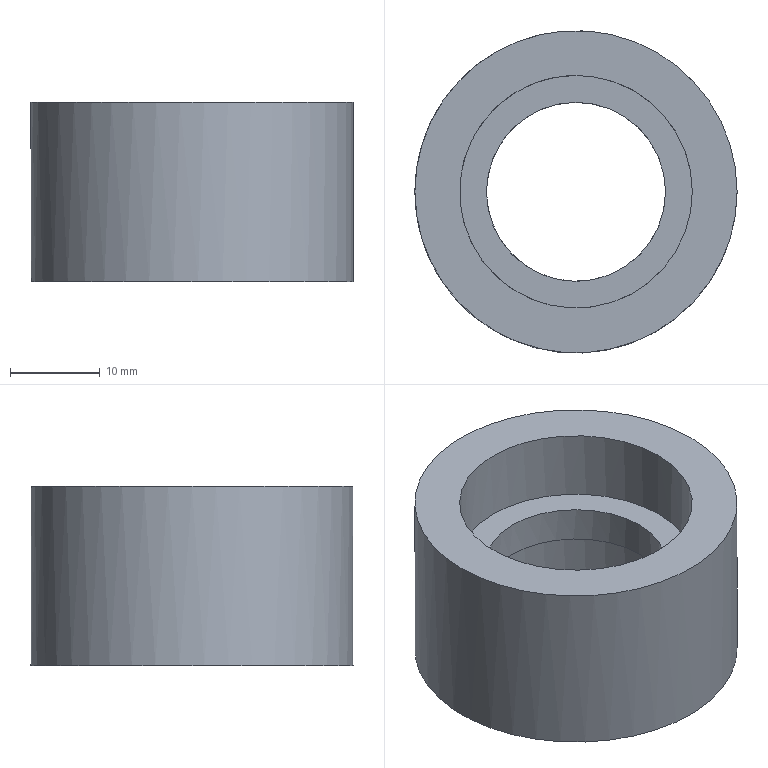Part | NX | features EXTRUDE 2, DATUM_CSYS 1, EXTRACT_DATUM_PLANE 1, SKETCH 1, UNITE 1 | 1 solid | 8 faces | box 36 x 36 x 20 mm | volume 10606 mm3 | cylinder 4 | plane 4 | commonest cylinder face diameters 26 x2 20 x1 36 x1
STEP:
#1=CARTESIAN_POINT('',(-13.,0.,-10.));
#2=VERTEX_POINT('',#1);
#3=CARTESIAN_POINT('',(0.,0.,-10.));
#4=DIRECTION('',(0.,0.,-1.));
#5=DIRECTION('',(-1.,0.,0.));
#6=AXIS2_PLACEMENT_3D('',#3,#4,#5);
#7=CIRCLE('',#6,13.);
#8=EDGE_CURVE('',#2,#2,#7,.T.);
#9=ORIENTED_EDGE('',*,*,#8,.T.);
#10=EDGE_LOOP('',(#9));
#11=FACE_BOUND('',#10,.T.);
#12=CARTESIAN_POINT('',(13.,0.,-2.));
#13=VERTEX_POINT('',#12);
#14=CARTESIAN_POINT('',(0.,0.,-2.));
#15=DIRECTION('',(0.,0.,1.));
#16=DIRECTION('',(1.,0.,0.));
#17=AXIS2_PLACEMENT_3D('',#14,#15,#16);
#18=CIRCLE('',#17,13.);
#19=EDGE_CURVE('',#13,#13,#18,.T.);
#20=ORIENTED_EDGE('',*,*,#19,.T.);
#21=EDGE_LOOP('',(#20));
#22=FACE_BOUND('',#21,.T.);
#23=CARTESIAN_POINT('',(0.,0.,-10.));
#24=DIRECTION('',(0.,0.,1.));
#25=DIRECTION('',(1.,0.,0.));
#26=AXIS2_PLACEMENT_3D('',#23,#24,#25);
#27=CYLINDRICAL_SURFACE('',#26,13.);
#28=ADVANCED_FACE('',(#11,#22),#27,.F.);
#29=CARTESIAN_POINT('',(-18.,0.,10.));
#30=VERTEX_POINT('',#29);
#31=CARTESIAN_POINT('',(0.,0.,10.));
#32=DIRECTION('',(0.,0.,1.));
#33=DIRECTION('',(-1.,0.,0.));
#34=AXIS2_PLACEMENT_3D('',#31,#32,#33);
#35=CIRCLE('',#34,18.);
#36=EDGE_CURVE('',#30,#30,#35,.T.);
#37=ORIENTED_EDGE('',*,*,#36,.F.);
#38=EDGE_LOOP('',(#37));
#39=FACE_BOUND('',#38,.T.);
#40=CARTESIAN_POINT('',(18.,0.,-10.));
#41=VERTEX_POINT('',#40);
#42=CARTESIAN_POINT('',(0.,0.,-10.));
#43=DIRECTION('',(0.,0.,1.));
#44=DIRECTION('',(1.,0.,0.));
#45=AXIS2_PLACEMENT_3D('',#42,#43,#44);
#46=CIRCLE('',#45,18.);
#47=EDGE_CURVE('',#41,#41,#46,.T.);
#48=ORIENTED_EDGE('',*,*,#47,.T.);
#49=EDGE_LOOP('',(#48));
#50=FACE_BOUND('',#49,.T.);
#51=CARTESIAN_POINT('',(0.,0.,-10.));
#52=DIRECTION('',(0.,0.,1.));
#53=DIRECTION('',(1.,0.,0.));
#54=AXIS2_PLACEMENT_3D('',#51,#52,#53);
#55=CYLINDRICAL_SURFACE('',#54,18.);
#56=ADVANCED_FACE('',(#39,#50),#55,.T.);
#57=CARTESIAN_POINT('',(-13.,0.,2.));
#58=VERTEX_POINT('',#57);
#59=CARTESIAN_POINT('',(0.,0.,2.));
#60=DIRECTION('',(0.,0.,1.));
#61=DIRECTION('',(-1.,0.,0.));
#62=AXIS2_PLACEMENT_3D('',#59,#60,#61);
#63=CIRCLE('',#62,13.);
#64=EDGE_CURVE('',#58,#58,#63,.T.);
#65=ORIENTED_EDGE('',*,*,#64,.F.);
#66=EDGE_LOOP('',(#65));
#67=FACE_BOUND('',#66,.T.);
#68=CARTESIAN_POINT('',(13.,0.,10.));
#69=VERTEX_POINT('',#68);
#70=CARTESIAN_POINT('',(0.,0.,10.));
#71=DIRECTION('',(0.,0.,-1.));
#72=DIRECTION('',(1.,0.,0.));
#73=AXIS2_PLACEMENT_3D('',#70,#71,#72);
#74=CIRCLE('',#73,13.);
#75=EDGE_CURVE('',#69,#69,#74,.T.);
#76=ORIENTED_EDGE('',*,*,#75,.F.);
#77=EDGE_LOOP('',(#76));
#78=FACE_BOUND('',#77,.T.);
#79=CARTESIAN_POINT('',(0.,0.,-10.));
#80=DIRECTION('',(0.,0.,1.));
#81=DIRECTION('',(1.,0.,0.));
#82=AXIS2_PLACEMENT_3D('',#79,#80,#81);
#83=CYLINDRICAL_SURFACE('',#82,13.);
#84=ADVANCED_FACE('',(#67,#78),#83,.F.);
#85=ORIENTED_EDGE('',*,*,#47,.F.);
#86=EDGE_LOOP('',(#85));
#87=FACE_BOUND('',#86,.T.);
#88=ORIENTED_EDGE('',*,*,#8,.F.);
#89=EDGE_LOOP('',(#88));
#90=FACE_BOUND('',#89,.T.);
#91=CARTESIAN_POINT('',(0.,0.,-10.));
#92=DIRECTION('',(0.,0.,1.));
#93=DIRECTION('',(1.,0.,0.));
#94=AXIS2_PLACEMENT_3D('',#91,#92,#93);
#95=PLANE('',#94);
#96=ADVANCED_FACE('',(#87,#90),#95,.F.);
#97=ORIENTED_EDGE('',*,*,#36,.T.);
#98=EDGE_LOOP('',(#97));
#99=FACE_BOUND('',#98,.T.);
#100=ORIENTED_EDGE('',*,*,#75,.T.);
#101=EDGE_LOOP('',(#100));
#102=FACE_BOUND('',#101,.T.);
#103=CARTESIAN_POINT('',(0.,0.,10.));
#104=DIRECTION('',(0.,0.,1.));
#105=DIRECTION('',(1.,0.,0.));
#106=AXIS2_PLACEMENT_3D('',#103,#104,#105);
#107=PLANE('',#106);
#108=ADVANCED_FACE('',(#99,#102),#107,.T.);
#109=CARTESIAN_POINT('',(-10.,0.,2.));
#110=VERTEX_POINT('',#109);
#111=CARTESIAN_POINT('',(0.,0.,2.));
#112=DIRECTION('',(0.,0.,-1.));
#113=DIRECTION('',(-1.,0.,0.));
#114=AXIS2_PLACEMENT_3D('',#111,#112,#113);
#115=CIRCLE('',#114,10.);
#116=EDGE_CURVE('',#110,#110,#115,.T.);
#117=ORIENTED_EDGE('',*,*,#116,.F.);
#118=EDGE_LOOP('',(#117));
#119=FACE_BOUND('',#118,.T.);
#120=CARTESIAN_POINT('',(10.,0.,-2.));
#121=VERTEX_POINT('',#120);
#122=CARTESIAN_POINT('',(0.,0.,-2.));
#123=DIRECTION('',(0.,0.,-1.));
#124=DIRECTION('',(1.,0.,0.));
#125=AXIS2_PLACEMENT_3D('',#122,#123,#124);
#126=CIRCLE('',#125,10.);
#127=EDGE_CURVE('',#121,#121,#126,.T.);
#128=ORIENTED_EDGE('',*,*,#127,.T.);
#129=EDGE_LOOP('',(#128));
#130=FACE_BOUND('',#129,.T.);
#131=CARTESIAN_POINT('',(0.,0.,-2.));
#132=DIRECTION('',(0.,0.,1.));
#133=DIRECTION('',(1.,0.,0.));
#134=AXIS2_PLACEMENT_3D('',#131,#132,#133);
#135=CYLINDRICAL_SURFACE('',#134,10.);
#136=ADVANCED_FACE('',(#119,#130),#135,.F.);
#137=ORIENTED_EDGE('',*,*,#19,.F.);
#138=EDGE_LOOP('',(#137));
#139=FACE_BOUND('',#138,.T.);
#140=ORIENTED_EDGE('',*,*,#127,.F.);
#141=EDGE_LOOP('',(#140));
#142=FACE_BOUND('',#141,.T.);
#143=CARTESIAN_POINT('',(0.,0.,-2.));
#144=DIRECTION('',(0.,0.,1.));
#145=DIRECTION('',(1.,0.,0.));
#146=AXIS2_PLACEMENT_3D('',#143,#144,#145);
#147=PLANE('',#146);
#148=ADVANCED_FACE('',(#139,#142),#147,.F.);
#149=ORIENTED_EDGE('',*,*,#64,.T.);
#150=EDGE_LOOP('',(#149));
#151=FACE_BOUND('',#150,.T.);
#152=ORIENTED_EDGE('',*,*,#116,.T.);
#153=EDGE_LOOP('',(#152));
#154=FACE_BOUND('',#153,.T.);
#155=CARTESIAN_POINT('',(0.,0.,2.));
#156=DIRECTION('',(0.,0.,1.));
#157=DIRECTION('',(1.,0.,0.));
#158=AXIS2_PLACEMENT_3D('',#155,#156,#157);
#159=PLANE('',#158);
#160=ADVANCED_FACE('',(#151,#154),#159,.T.);
#161=CLOSED_SHELL('',(#28,#56,#84,#96,#108,#136,#148,#160));
#162=MANIFOLD_SOLID_BREP('',#161);
#163=(LENGTH_UNIT()NAMED_UNIT(*)SI_UNIT(.MILLI.,.METRE.));
#164=UNCERTAINTY_MEASURE_WITH_UNIT(LENGTH_MEASURE(0.00001),#163,'','');
#165=(NAMED_UNIT(*)PLANE_ANGLE_UNIT()SI_UNIT($,.RADIAN.));
#166=(NAMED_UNIT(*)SI_UNIT($,.STERADIAN.)SOLID_ANGLE_UNIT());
#167=(GEOMETRIC_REPRESENTATION_CONTEXT(3)GLOBAL_UNCERTAINTY_ASSIGNED_CONTEXT((#164))GLOBAL_UNIT_ASSIGNED_CONTEXT((#163,#165,#166))REPRESENTATION_CONTEXT('',''));
#168=ADVANCED_BREP_SHAPE_REPRESENTATION('',(#162),#167);